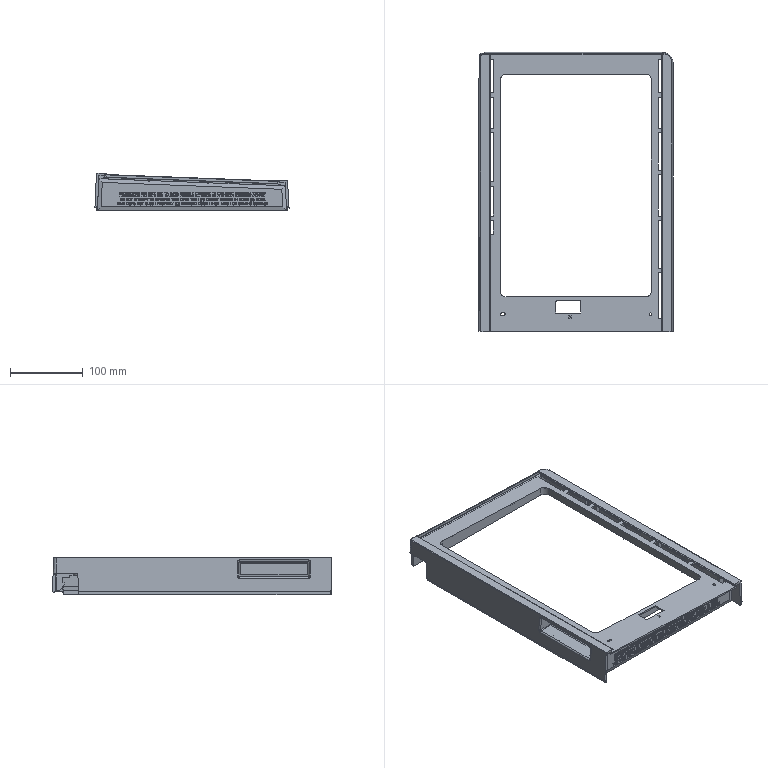Part | Creo | 1 solid | 2523 faces | box 267.224 x 384.325 x 51.211 mm | volume 272728 mm3 | plane 1903 | other 472 | cylinder 119 | spline 16 | sphere 8 | cone 4 | torus 1 | commonest cylinder face diameters 2.009 x47 1.004 x14 10.118 x10 8.036 x8 4.018 x7 5.022 x5